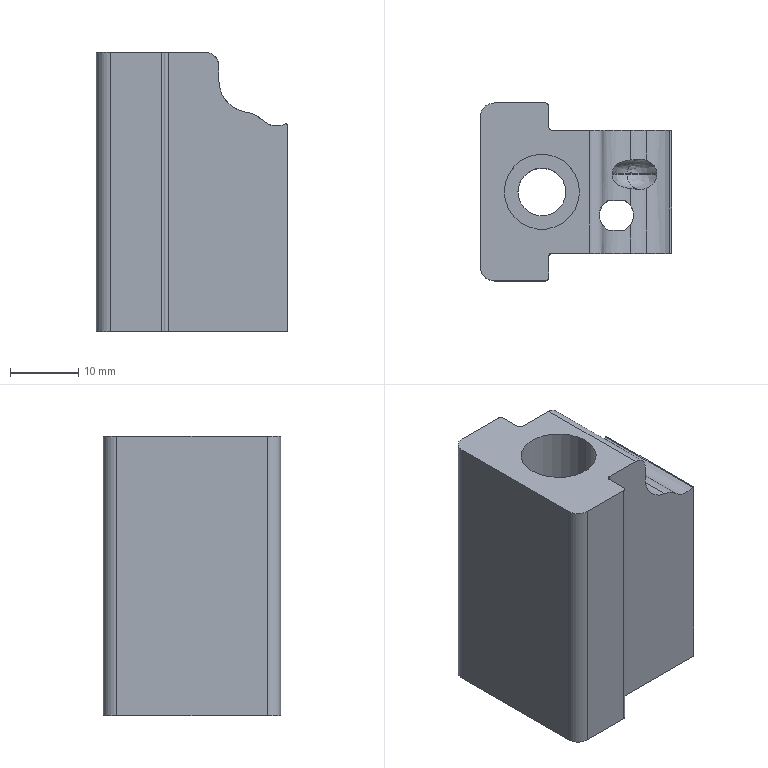Part | 1 solid | 45 faces | box 28 x 26 x 40.95 mm | volume 19091 mm3 | cylinder 22 | plane 17 | spline 6 | commonest cylinder face diameters 1 x4 4 x3 5 x2 7 x2 8.2 x2 9 x2